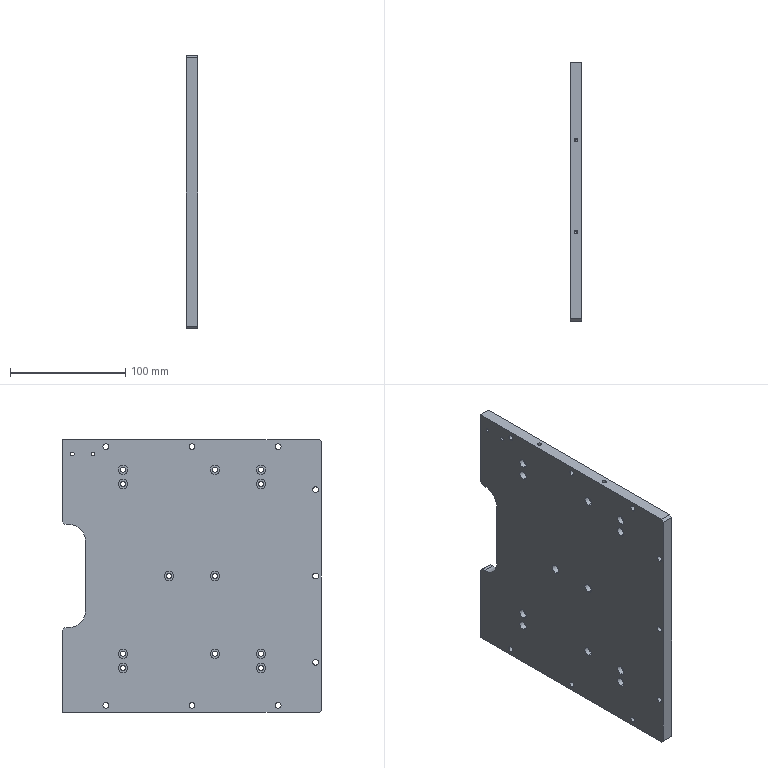Part | SolidWorks | features HoleWzd 6, Chamfer 2, MirrorPattern 2, MoveFace 2, Extrusion 1, ICE 1 | 1 solid | 114 faces | box 10 x 225 x 237 mm | volume 510039 mm3 | cylinder 80 | plane 26 | cone 8 | commonest cylinder face diameters 4.3 x24 8 x24 5 x18 3.3 x12 30 x2